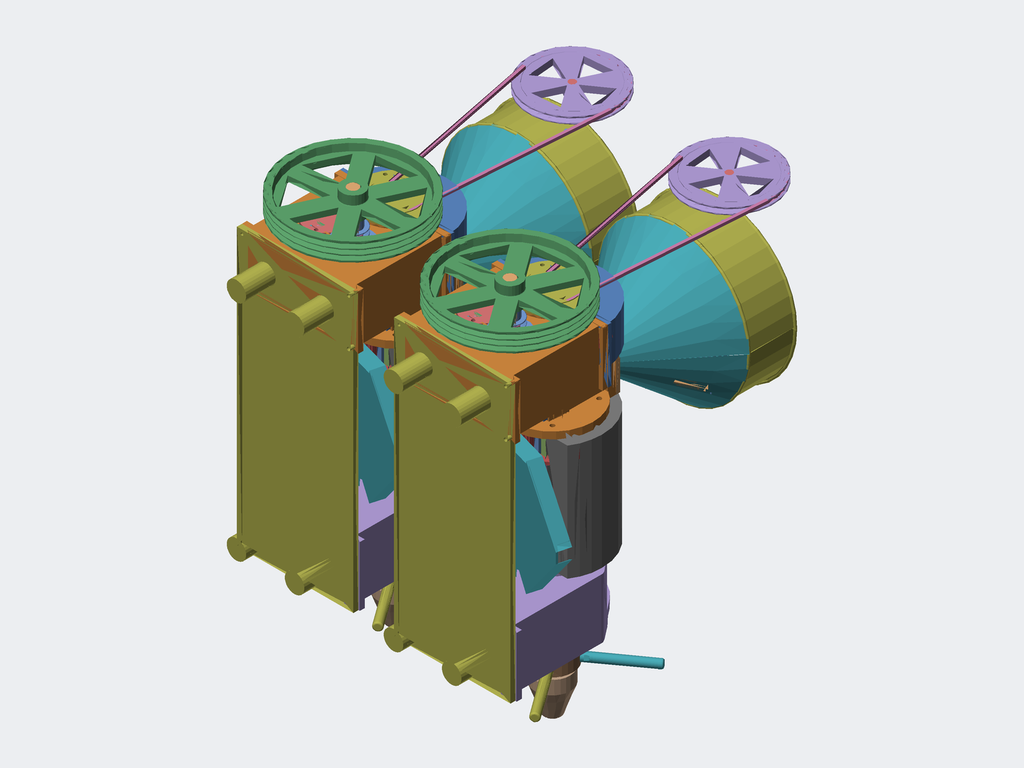Assembly | SolidWorks | 63 different items | 150 placed
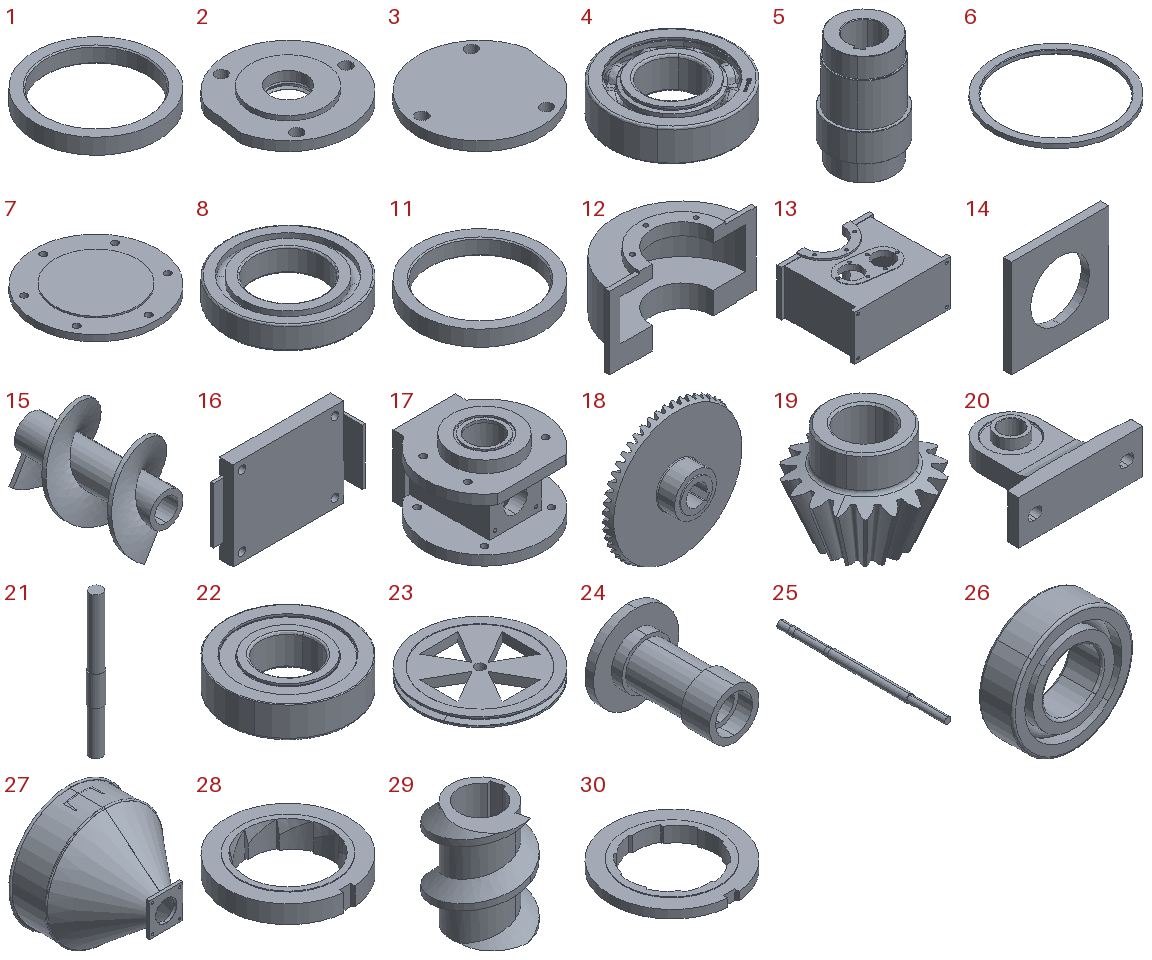Parts list (item | quantity | size | volume | features):
1 | x2 | 55 x 55 x 7 mm | 5462 mm3 | features Revolution 1
2 | x2 | 130.573 x 132 x 19 mm | 150304 mm3 | features HoleWzd 2, Revolution 2, BaseBody 1, Extrusion 1
3 | x6 | 130.573 x 132 x 14 mm | 142005 mm3 | features HoleWzd 2, Extrusion 1, Revolution 1
4 | x4 | 90 x 90 x 23 mm | 82930 mm3 | features BaseBody 14
5 | x2 | 110 x 110 x 178 mm | 973022 mm3 | features BaseBody 1
6 | x1 | 114 x 114 x 4 mm | 9333 mm3 | features Revolution 1
7 | x2 | 240 x 240 x 17.5 mm | 563209 mm3 | features ICE 3, HoleWzd 2, Revolution 1
8 | x4 | 170 x 170 x 32 mm | 443055 mm3 | features BaseBody 1
9 | x2 | - | - | features BaseBody 1
10 | x2 | - | - | features BaseBody 1
11 | x4 | 55 x 55 x 7 mm | 5462 mm3 | features Revolution 1
12 | x2 | 410 x 187 x 210 mm | 2846531 mm3 | features ICE 6, HoleWzd 2, Extrusion 1, RevCut 1
13 | x2 | 430 x 352 x 210 mm | 7645856 mm3 | features ICE 16, HoleWzd 12, Extrusion 1, Fillet 1
14 | x2 | 120 x 10 x 120 mm | 103285 mm3 | features Extrusion 1
15 | x2 | 82 x 130 x 82 mm | 90947 mm3 | features ICE 3, BaseBody 1, HoleWzd 1
16 | x2 | 144 x 31 x 100 mm | 183212 mm3 | features BaseBody 1, Extrusion 1
17 | x2 | 300 x 305 x 198 mm | 5533662 mm3 | features HoleWzd 8, ICE 6, Revolution 2, Extrusion 1
18 | x2 | 160.088 x 42.208 x 160.125 mm | 285045 mm3 | features BaseBody 1
19 | x2 | 61.792 x 61.935 x 51.071 mm | 51754 mm3 | features BaseBody 1
20 | x4 | 142 x 118.08 x 50 mm | 239637 mm3 | features ICE 3, Revolution 3, Fillet 2, BaseBody 1, Chamfer 1, HoleWzd 1
21 | x2 | 28 x 28 x 290 mm | 149846 mm3 | features Revolution 1
22 | x4 | 90 x 90 x 23 mm | 84067 mm3 | features BaseBody 14
23 | x2 | 320 x 320 x 39 mm | 1356183 mm3 | features Fillet 3, ICE 2, Revolution 2, BaseBody 1, HoleWzd 1, RevCut 1
24 | x2 | 120 x 165 x 120 mm | 395872 mm3 | features Revolution 1
25 | x2 | - | - | features ICE 3, RefSurface 1, Revolution 1
26 | x2 | 52 x 15 x 52 mm | 20902 mm3 | features BaseBody 1
27 | x2 | 572 x 466.152 x 572 mm | 1942635 mm3 | features BaseBody 4
28 | x4 | 150 x 149.673 x 31.5 mm | 269452 mm3 | features BaseBody 1, ICE 1
29 | x6 | 95 x 95 x 120 mm | 282927 mm3 | features BaseBody 1, ICE 1, RevCut 1
30 | x6 | 150 x 149.673 x 18.5 mm | 146475 mm3 | features BaseBody 1, ICE 1
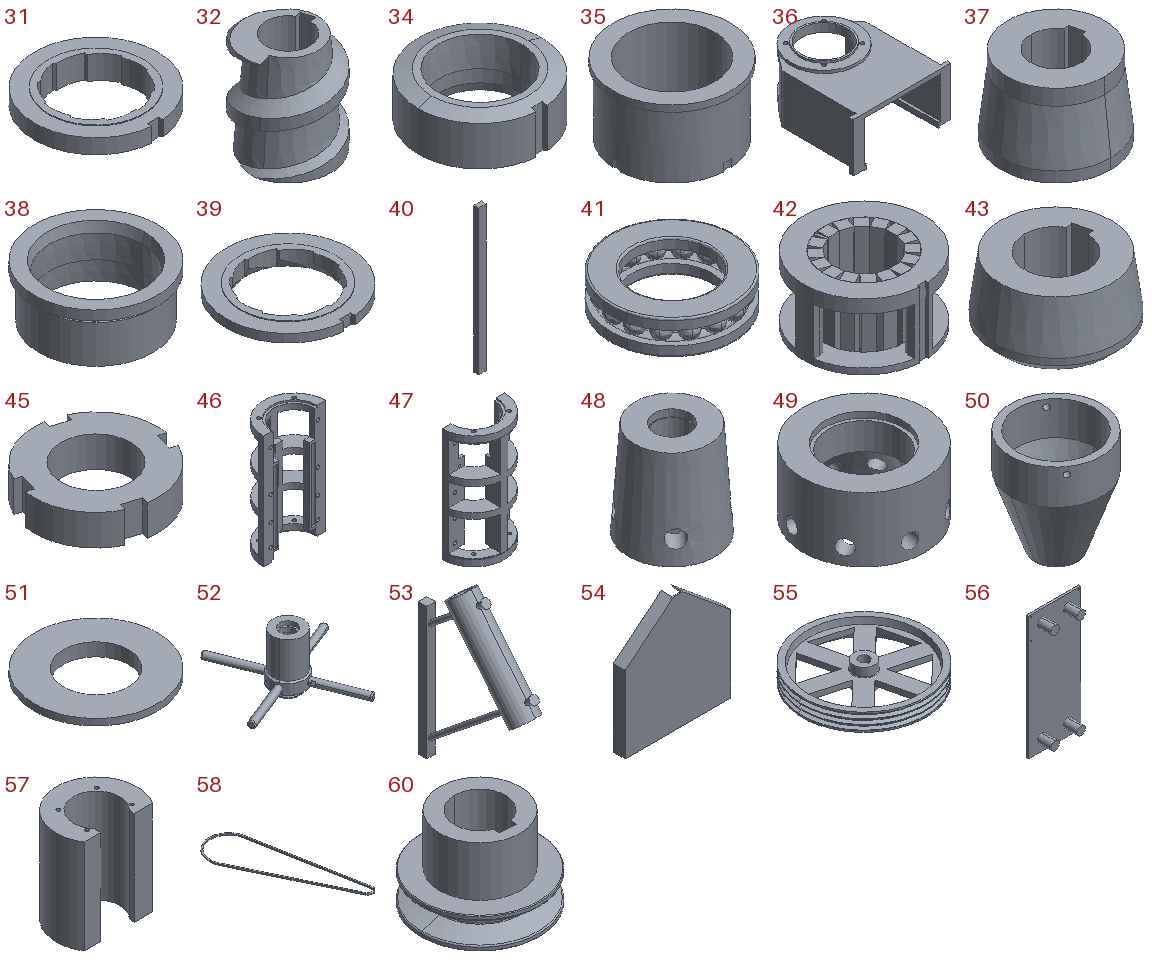31 | x4 | 150 x 149.673 x 28.6 mm | 237488 mm3 | features BaseBody 1, ICE 1
32 | x2 | 95.001 x 95.001 x 109 mm | 363521 mm3 | features BaseBody 1, ICE 1, RevCut 1
33 | x2 | - | - | features BaseBody 1
34 | x2 | 150 x 149.673 x 58.5 mm | 537765 mm3 | features BaseBody 1, ICE 1
35 | x2 | 185 x 185 x 110 mm | 1098272 mm3 | features ICE 5, HoleWzd 1, Revolution 1
36 | x2 | 440 x 502 x 295 mm | 8777626 mm3 | features ICE 17, Fillet 4, HoleWzd 3, Cut 1, Extrusion 1, Revolution 1
37 | x2 | 106 x 106 x 75 mm | 445446 mm3 | features ICE 1, RevCut 1, Revolution 1
38 | x2 | 130 x 130 x 55 mm | 211427 mm3 | features Revolution 1
39 | x4 | 150 x 149.673 x 18.5 mm | 145659 mm3 | features BaseBody 1, ICE 1
40 | x2 | 14 x 9 x 265 mm | 33390 mm3 | features Extrusion 1
41 | x2 | 73 x 73 x 20 mm | 37195 mm3 | features BaseBody 1
42 | x2 | 200 x 199.755 x 123 mm | 1515679 mm3 | features BaseBody 18
43 | x2 | 95 x 95 x 50 mm | 226212 mm3 | features ICE 1, RevCut 1, Revolution 1
44 | x2 | - | - | features BaseBody 1
45 | x2 | 80 x 80 x 20 mm | 64249 mm3 | features Extrusion 1
46 | x1 | 300 x 150 x 550 mm | 5053436 mm3 | features ICE 6, HoleWzd 3, RevCut 3, Revolution 1
47 | x1 | 300 x 150 x 550 mm | 5063192 mm3 | features ICE 19, HoleWzd 4, RevCut 4, BaseBody 1
48 | x2 | 125 x 125 x 135 mm | 1121518 mm3 | features HoleWzd 7, Revolution 1
49 | x2 | 205 x 205 x 108 mm | 1920095 mm3 | features 3DProfileFeature 8, HoleWzd 8, RevCut 1, Revolution 1
50 | x2 | 130 x 130 x 150 mm | 468175 mm3 | features HoleWzd 2, 3DProfileFeature 1, Fillet 1, Revolution 1
51 | x2 | 95 x 95 x 10 mm | 41529 mm3 | features Revolution 1
52 | x2 | 555.753 x 555.753 x 240 mm | 3106019 mm3 | features BaseBody 5
53 | x2 | 45 x 200.096 x 286.61 mm | 222734 mm3 | features ICE 7, Cut 1, Extrusion 1
54 | x2 | 425.348 x 48 x 468.238 mm | 1599795 mm3 | features Cut 1, Extrusion 1, Shell 1
55 | x2 | 470 x 470 x 87 mm | 3518075 mm3 | features ICE 5, Fillet 4, BaseBody 1, RevCut 1
56 | x2 | 430 x 128 x 1020 mm | 9620878 mm3 | features Extrusion 1, ICE 1
57 | x2 | 364.306 x 280.408 x 426 mm | 21434816 mm3 | features Extrusion 1
58 | x2 | 465.093 x 1023 x 10 mm | 233862 mm3 | features ExtruThin 1
59 | x2 | - | - | features ICE 5, BaseBody 1, RefSurface 1, Revolution 1
60 | x2 | 88 x 88 x 60 mm | 133834 mm3 | features Fillet 2, ICE 2, Chamfer 1, RevCut 1, Revolution 1
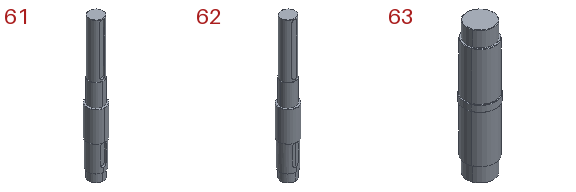61 | x2 | 50 x 50 x 384 mm | 534684 mm3 | features BaseBody 1
62 | x1 | - | - | features ICE 6, RefSurface 2, Chamfer 1, Revolution 1
63 | x2 | 48 x 48 x 200 mm | 297463 mm3 | features BaseBody 1
Mates (type | each side: item.copy, entity, surface, feature):
Coincident | 55.1 face plane Boss-Extrude1 | 61.1 edge
Concentric | 55.1 face cylinder Cut-Revolve1 | 61.1 face cylinder Gearbox assembly-1/1-shaft-1/1-shaft-1-solid1
Parallel | 55.1 face plane Cut-Extrude1 | 61.1 face plane Gearbox assembly-1/1-shaft-1/1-shaft-1-solid1
Concentric | 61.1 face cylinder Gearbox assembly-1/1-shaft-1/1-shaft-1-solid1 | 60.1 face cylinder Cut-Revolve1
Parallel | 61.1 face plane Gearbox assembly-1/1-shaft-1/1-shaft-1-solid1 | 60.1 face plane Cut-Extrude1
Coincident | 55.1 face plane Boss-Extrude2 | 60.1 face plane Boss-Extrude1
Concentric | 13.1 face cylinder M80 clearance hole1 | 61.1 face cylinder Gearbox assembly-1/1-shaft-1/1-shaft-1-solid1
Coincident | 13.1 face plane Boss-Extrude12 | 2.1 face plane Boss-Extrude1
Concentric | 13.1 face cylinder Ø12.0 (12) diameter hole5 | 2.1 face cylinder Ø12.5 (12.5) Diameter Hole1 | 2 times
Concentric | 13.1 face cylinder M80 clearance hole2 | 4.1 face cylinder Gearbox assembly-1/1-shaft-1/1-bearing-gearbox 6308-1-solid11
Coincident | 13.1 face plane Boss-Extrude14 | 4.1 face plane Gearbox assembly-1/1-shaft-1/1-bearing-gearbox 6308-1-solid6
Coincident | 61.1 face plane Gearbox assembly-1/1-shaft-1/1-shaft-1-solid1 | 4.1 face plane Gearbox assembly-1/1-shaft-1/1-bearing-gearbox 6308-1-solid11
Concentric | 13.1 face cylinder M80 clearance hole2 | 4.2 face cylinder Gearbox assembly-1/1-shaft-1/1-bearing-gearbox 6308-1-solid11
Coincident | 13.1 face plane Boss-Extrude13 | 4.2 face plane Gearbox assembly-1/1-shaft-1/1-bearing-gearbox 6308-1-solid6
Coincident | 10.1 face plane Gearbox assembly-1/1-shaft-1/1-small spur gear-1-solid1 | 61.1 face plane Gearbox assembly-1/1-shaft-1/1-shaft-1-solid1
Parallel | 10.1 face plane Gearbox assembly-1/1-shaft-1/1-small spur gear-1-solid1 | 61.1 face plane Gearbox assembly-1/1-shaft-1/1-shaft-1-solid1
Concentric | 10.1 face cylinder Gearbox assembly-1/1-shaft-1/1-small spur gear-1-solid1 | 61.1 face cylinder Gearbox assembly-1/1-shaft-1/1-shaft-1-solid1
Coincident | 1.1 face plane Revolve1 | 4.2 face plane Gearbox assembly-1/1-shaft-1/1-bearing-gearbox 6308-1-solid6
Concentric | 61.1 face cylinder Gearbox assembly-1/1-shaft-1/1-shaft-1-solid1 | 1.1 face cylinder Revolve1
Coincident | 13.1 face plane Boss-Extrude9 | 3.1 face plane Boss-Extrude1
Concentric | 13.1 face cylinder Ø12.0 (12) diameter hole4 | 3.1 face cylinder Ø12.5 (12.5) Diameter Hole1 | 2 times
Concentric | 13.1 face cylinder M80 clearance hole1 | 63.1 face cylinder Gearbox assembly-1/2-shaft-1/2-shaft-1-solid1
Coincident | 13.1 face plane Boss-Extrude12 | 63.1 face plane Gearbox assembly-1/2-shaft-1/2-shaft-1-solid1
Concentric | 13.1 face cylinder M80 clearance hole1 | 22.1 face cylinder Gearbox assembly-1/2-shaft-1/2-bearing-gearbox 6308-1-solid11
Coincident | 13.1 face plane Boss-Extrude14 | 22.1 face plane Gearbox assembly-1/2-shaft-1/2-bearing-gearbox 6308-1-solid6
Concentric | 13.1 face cylinder M80 clearance hole2 | 22.2 face cylinder Gearbox assembly-1/2-shaft-1/2-bearing-gearbox 6308-1-solid11
Coincident | 13.1 face plane Boss-Extrude13 | 22.2 face plane Gearbox assembly-1/2-shaft-1/2-bearing-gearbox 6308-1-solid6
Coincident | 13.1 face plane Boss-Extrude12 | 3.2 face plane Boss-Extrude1
Concentric | 13.1 face cylinder Ø12.0 (12) diameter hole5 | 3.2 face cylinder Ø12.5 (12.5) Diameter Hole1 | 2 times
Coincident | 13.1 face plane Boss-Extrude9 | 3.3 face plane Boss-Extrude1
Concentric | 13.1 face cylinder Ø12.0 (12) diameter hole4 | 3.3 face cylinder Ø12.5 (12.5) Diameter Hole1 | 2 times
Concentric | 63.1 face cylinder Gearbox assembly-1/2-shaft-1/2-shaft-1-solid1 | 11.1 face cylinder Revolve1
Coincident | 11.1 face plane Revolve1 | 22.2 face plane Gearbox assembly-1/2-shaft-1/2-bearing-gearbox 6308-1-solid11
Concentric | 63.1 face cylinder Gearbox assembly-1/2-shaft-1/2-shaft-1-solid1 | 9.1 face cylinder Gearbox assembly-1/2-shaft-1/2-large spur gear-1-solid1
Parallel | 63.1 face plane Gearbox assembly-1/2-shaft-1/2-shaft-1-solid1 | 9.1 face plane Gearbox assembly-1/2-shaft-1/2-large spur gear-1-solid1
Coincident | 11.1 face plane Revolve1 | 9.1 face plane Gearbox assembly-1/2-shaft-1/2-large spur gear-1-solid1
Coincident | 22.1 face plane Gearbox assembly-1/2-shaft-1/2-bearing-gearbox 6308-1-solid11 | 11.2 face plane Revolve1
Coincident | 44.1 face plane Gearbox assembly-1/2-shaft-1/2-small spur gear-1-solid1 | 11.2 face plane Revolve1
Concentric | 63.1 face cylinder Gearbox assembly-1/2-shaft-1/2-shaft-1-solid1 | 44.1 face cylinder Gearbox assembly-1/2-shaft-1/2-small spur gear-1-solid1
Parallel | 63.1 face plane Gearbox assembly-1/2-shaft-1/2-shaft-1-solid1 | 44.1 face plane Gearbox assembly-1/2-shaft-1/2-small spur gear-1-solid1
Coincident | 13.1 face plane Boss-Extrude6 | 7.1 face plane Revolve1
Concentric | 13.1 face cylinder Hole1 | 7.1 face cylinder M90 counterbore hole1
Concentric | 13.1 face cylinder Ø12.0 (12) diameter hole1 | 7.1 face cylinder Ø12.5 (12.5) Diameter Hole1
Coincident | 13.1 face plane Cut-Extrude1 | 8.1 face plane Gearbox assembly-1/3-shaft-2/3-bearing 6219-1-solid1
Concentric | 13.1 face cylinder Hole1 | 8.1 face cylinder Gearbox assembly-1/3-shaft-2/3-bearing 6219-1-solid1
Concentric | 13.1 face cylinder Hole2 | 8.2 face cylinder Gearbox assembly-1/3-shaft-2/3-bearing 6219-1-solid1
Coincident | 13.1 face plane Cut-Extrude1 | 8.2 face plane Gearbox assembly-1/3-shaft-2/3-bearing 6219-1-solid1
Concentric | 5.1 face cylinder Gearbox assembly-1/3-shaft-2/3-shaft-1-solid1 | 8.1 face cylinder Gearbox assembly-1/3-shaft-2/3-bearing 6219-1-solid1
Coincident | 5.1 face plane Gearbox assembly-1/3-shaft-2/3-shaft-1-solid1 | 8.2 face plane Gearbox assembly-1/3-shaft-2/3-bearing 6219-1-solid1
Concentric | 33.1 face cylinder Gearbox assembly-1/3-shaft-2/3-large spur gear-1-solid1 | 5.1 face cylinder Gearbox assembly-1/3-shaft-2/3-shaft-1-solid1
Parallel | 33.1 face plane Gearbox assembly-1/3-shaft-2/3-large spur gear-1-solid1 | 5.1 face plane Gearbox assembly-1/3-shaft-2/3-shaft-1-solid1
Coincident | 33.1 face plane Gearbox assembly-1/3-shaft-2/3-large spur gear-1-solid1 | 5.1 face plane Gearbox assembly-1/3-shaft-2/3-shaft-1-solid1
GearDim | 33.1 select_type:24 | 44.1 select_type:24
Coincident | 12.1 face plane Boss-Extrude1 | 13.1 face plane Boss-Extrude4
Coincident | 12.1 face plane Boss-Extrude1 | 13.1 face plane Boss-Extrude2
Coincident | 12.1 face plane Boss-Extrude1 | 13.1 face plane Boss-Extrude5
Coincident | 20.1 face plane Input3 | 27.1 face plane Hopper-1/Hopper-channel steel 14a-1-solid1
Concentric | 20.1 face cylinder Input3 | 27.1 face cylinder Hopper-1/Hopper-channel steel 14a-1-solid1 | 2 times
Parallel | 20.1 face cylinder Input3 | 27.1 face cylinder Hopper-1/Hopper-channel steel 14a-1-solid1
Coincident | 27.1 face plane Hopper-1/Hopper-channel steel 14a-1-solid1 | 20.2 face plane Input3
Concentric | 27.1 face cylinder Hopper-1/Hopper-channel steel 14a-1-solid1 | 20.2 face cylinder Input3 | 2 times
Concentric | 21.1 face cylinder Revolve1 | 20.2 face cylinder Ø25.0 (25) diameter hole1
Coincident | 21.1 face plane Revolve1 | 20.2 face plane Revolve3
Concentric | 21.1 face cylinder Revolve1 | 23.1 face cylinder Ø25.0 (25) diameter hole1
Coincident | 21.1 face plane Revolve1 | 23.1 face plane Cut-Revolve1
Coincident | 21.1 select_type:24 | 23.1 select_type:24
Coincident | 17.1 face plane Boss-Extrude4 | 27.1 face plane Hopper-1/Hopper-base-1-solid1
Concentric | 17.1 face cylinder Ø10.0 (10) diameter hole1 | 27.1 face cylinder Hopper-1/Hopper-base-1-solid1 | 2 times
Coincident | 16.1 face plane Input3 | 17.1 face plane Boss-Extrude2
Concentric | 16.1 face cylinder Input3 | 17.1 face cylinder Ø8.0 (8) diameter hole1 | 2 times
Concentric | 25.1 face cylinder Revolve1 | 27.1 face cylinder Hopper-1/Hopper-channel steel 14a-1-solid1
Coincident | 18.1 face plane Hopper-1/Hopper-bevel gear assembly-1/Hopper-bevel gear-large gear-1-solid1 | 25.1 face plane Boss-Extrude1
Concentric | 18.1 face cylinder Hopper-1/Hopper-bevel gear assembly-1/Hopper-bevel gear-large gear-1-solid1 | 25.1 face cylinder Boss-Extrude1
Parallel | 18.1 face plane Hopper-1/Hopper-bevel gear assembly-1/Hopper-bevel gear-large gear-1-solid1 | 25.1 face plane Cut-Extrude1
Coincident | 14.1 face plane Boss-Extrude1 | 27.1 face plane Hopper-1/Hopper-channel steel 14a-1-solid1
Parallel | 14.1 edge | 27.1 edge
Concentric | 14.1 face cylinder Boss-Extrude1 | 27.1 face cylinder Hopper-1/Hopper-channel steel 14a-1-solid1
Coincident | 24.1 face plane Revolve1 | 14.1 face plane Boss-Extrude1
Concentric | 24.1 face cylinder Revolve1 | 14.1 face cylinder Boss-Extrude1
Concentric | 21.1 face cylinder Revolve1 | 19.1 face cylinder Hopper-1/Hopper-bevel gear assembly-1/Hopper-bevel gear-small gear-1-solid1
Coincident | 21.1 face plane Revolve1 | 19.1 face plane Hopper-1/Hopper-bevel gear assembly-1/Hopper-bevel gear-small gear-1-solid1
Coincident | 18.1 face plane Hopper-1/Hopper-bevel gear assembly-1/Hopper-bevel gear-large gear-1-solid1 | 24.1 face plane Revolve1
Concentric | 25.1 face cylinder Revolve1 | 26.1 face cylinder Hopper-1/Hopper-auger-1/Hopper-bearing 6205-RS-1-solid1
Coincident | 24.1 face plane Revolve1 | 26.1 face plane Hopper-1/Hopper-auger-1/Hopper-bearing 6205-RS-1-solid1
Concentric | 25.1 face cylinder Boss-Extrude2 | 15.1 face cylinder Ø22.0 (22) diameter hole1
Coincident | 25.1 face plane Revolve1 | 15.1 face plane Boss-Extrude2
Concentric | 8.2 face cylinder Gearbox assembly-1/3-shaft-2/3-bearing 6219-1-solid1 | 17.1 face cylinder M80 counterbore hole1
Coincident | 12.1 face plane Boss-Extrude2 | 17.1 face plane Boss-Extrude3
Concentric | 13.1 face cylinder Ø16.0 (16) diameter hole1 | 17.1 face cylinder Ø16.5 (16.5) diameter hole1
GearDim | 19.1 select_type:24 | 18.1 select_type:24
Coincident | 21.1 select_type:24 | 19.1 select_type:24
Concentric | 5.1 face cylinder Gearbox assembly-1/3-shaft-2/3-shaft-1-solid1 | 59.1 face cylinder Boss-Extrude4 | 2 times
Parallel | 5.1 edge | 59.1 select_type:24
Coincident | 51.1 face plane Revolve1 | 59.1 face plane Boss-Extrude4
Concentric | 51.1 face cylinder Revolve1 | 59.1 face cylinder Boss-Extrude3
Concentric | 32.1 face cylinder Cut-Revolve1 | 59.1 face cylinder Boss-Extrude3
Concentric | 29.1 face cylinder Cut-Revolve1 | 59.1 face cylinder Boss-Extrude3
Coincident | 51.1 face plane Revolve1 | 29.1 face plane Input3
Concentric | 59.1 face cylinder Boss-Extrude3 | 29.2 face cylinder Cut-Revolve1
Parallel | 29.1 edge | 59.1 select_type:24
Coincident | 29.1 face plane Input3 | 29.2 face plane Input3
Lock | 29.1 select_type:0 | 29.2 select_type:0
Concentric | 59.1 face cylinder Boss-Extrude3 | 29.3 face cylinder Cut-Revolve1
Coincident | 29.2 face plane Input3 | 29.3 face plane Input3
Lock | 29.2 select_type:0 | 29.3 select_type:0
Coincident | 32.1 face plane Input3 | 29.3 face plane Input3
Lock | 32.1 select_type:0 | 29.3 select_type:0
Concentric | 43.1 face cylinder Cut-Revolve1 | 59.1 face cylinder Boss-Extrude3
Coincident | 32.1 face plane Input3 | 43.1 face plane Revolve1
Parallel | 43.1 edge | 59.1 select_type:24
Concentric | 38.1 face cone Revolve1 | 59.1 face cylinder Boss-Extrude3
Coincident | 38.1 face plane Revolve1 | 43.1 face plane Revolve1
Concentric | 37.1 face cylinder Cut-Revolve1 | 59.1 face cylinder Boss-Extrude1
Coincident | 37.1 face plane Revolve1 | 43.1 face plane Revolve1
Concentric | 48.1 face cylinder M42 counterbore hole1 | 59.1 face cylinder Boss-Extrude1
Coincident | 37.1 face plane Revolve1 | 48.1 face plane Revolve1
Coincident | 38.1 face plane Revolve1 | 49.1 face plane Revolve1
Concentric | 38.1 face cylinder Revolve1 | 49.1 face cylinder Cut-Revolve1
Concentric | 41.1 face cylinder Press screw-1/Press screw-GB/T 301-1995[thrust ball bearing[51000]51209]-1-solid1 | 59.1 face cylinder Revolve1
Concentric | 52.1 face cylinder Press screw-1/Press screw-adjusting screw-1-solid1 | 59.1 face cylinder Input3
Coincident | 48.1 face plane Revolve1 | 52.1 face plane Press screw-1/Press screw-adjusting screw-1-solid1
Coincident | 52.1 face plane Press screw-1/Press screw-adjusting screw-1-solid1 | 41.1 face plane Press screw-1/Press screw-GB/T 301-1995[thrust ball bearing[51000]51209]-1-solid1
Concentric | 45.1 face cylinder Boss-Extrude1 | 59.1 face cylinder Revolve1
Coincident | 41.1 face plane Press screw-1/Press screw-GB/T 301-1995[thrust ball bearing[51000]51209]-1-solid1 | 45.1 face plane Boss-Extrude1
Concentric | 50.1 face cylinder M100 clearance hole1 | 59.1 face cylinder Revolve1
Coincident | 52.1 edge | 50.1 face plane Revolve1
Concentric | 35.1 face cylinder Hole1 | 52.1 face cylinder Press screw-1/Press screw-adjusting screw-1-solid1
Concentric | 35.1 face cylinder Boss-Extrude1 | 36.1 face cylinder Hole2
Lock | 35.1 select_type:0 | 52.1 select_type:0
Coincident | 35.1 face plane Cut-Extrude3 | 36.1 face plane M10 counterbore hole1
Coincident | 17.1 face plane Boss-Extrude3 | 51.1 face plane Revolve1
Coincident | 17.1 face plane Revolve1 | 42.1 face plane Oil discharge bar-1/Oil discharge bar-strip bar support-1-solid1
Concentric | 17.1 face cylinder M80 counterbore hole1 | 42.1 face cone Oil discharge bar-1/Oil discharge bar-strip bar support-1-solid1
Coincident | 25.1 select_type:24 | 15.1 select_type:24
Coincident | 42.1 face plane Oil discharge bar-1/Oil discharge bar-strip bar support-1-solid1 | 28.1 face plane Three-stage round bar-1/Round bar set-No.4 round bar-1-solid1
Concentric | 59.1 face cylinder Boss-Extrude4 | 28.1 edge
Concentric | 59.1 face cylinder Boss-Extrude4 | 31.1 edge
Concentric | 8.2 edge | 30.1 edge
Concentric | 59.1 face cylinder Boss-Extrude4 | 39.1 edge
Concentric | 59.1 face cylinder Boss-Extrude4 | 34.1 edge
Coincident | 31.1 face plane Three-stage round bar-1/Round bar set-No.3 round bar-2-solid1 | 28.1 face plane Three-stage round bar-1/Round bar set-No.4 round bar-1-solid1 | 2 times
Coincident | 31.1 face plane Cut-Extrude1 | 30.1 face plane Three-stage round bar-1/Round bar set-No.2 round bar-1-solid1
Coincident | 30.1 face plane Cut-Extrude1 | 39.1 face plane Three-stage round bar-1/Round bar set-No.2 round bar outer-1-solid1
Concentric | 59.1 face cylinder Boss-Extrude4 | 30.2 edge
Concentric | 59.1 face cylinder Boss-Extrude4 | 31.2 edge
Concentric | 59.1 face cylinder Boss-Extrude4 | 39.2 edge
Concentric | 59.1 face cylinder Boss-Extrude4 | 28.2 edge
Coincident | 39.1 face plane Cut-Extrude1 | 28.2 face plane Three-stage round bar-1/Round bar set-No.4 round bar-1-solid1
Coincident | 31.2 face plane Three-stage round bar-1/Round bar set-No.3 round bar-2-solid1 | 28.2 face plane Three-stage round bar-1/Round bar set-No.4 round bar-1-solid1 | 2 times
Coincident | 31.2 face plane Cut-Extrude1 | 30.2 face plane Three-stage round bar-1/Round bar set-No.2 round bar-1-solid1
Coincident | 30.2 face plane Cut-Extrude1 | 39.2 face plane Three-stage round bar-1/Round bar set-No.2 round bar outer-1-solid1
Concentric | 59.1 face cylinder Boss-Extrude4 | 30.3 edge
Coincident | 39.2 face plane Cut-Extrude1 | 30.3 face plane Three-stage round bar-1/Round bar set-No.2 round bar-1-solid1
Coincident | 34.1 face plane Three-stage round bar-1/Round bar set-No.5 round bar-1-solid1 | 30.3 face plane Cut-Extrude1
Parallel | 42.1 face plane Oil discharge bar-1/Oil discharge bar-strip bar support-1-solid1 | 28.1 face plane Three-stage round bar-1/Round bar set-No.4 round bar-1-solid1
Coincident | 31.1 face plane Three-stage round bar-1/Round bar set-No.3 round bar-2-solid1 | 30.1 face plane Three-stage round bar-1/Round bar set-No.2 round bar-1-solid1
Coincident | 30.1 face plane Three-stage round bar-1/Round bar set-No.2 round bar-1-solid1 | 39.1 face plane Three-stage round bar-1/Round bar set-No.2 round bar outer-1-solid1
Coincident | 39.1 face plane Three-stage round bar-1/Round bar set-No.2 round bar outer-1-solid1 | 28.2 face plane Three-stage round bar-1/Round bar set-No.4 round bar-1-solid1
Coincident | 31.2 face plane Three-stage round bar-1/Round bar set-No.3 round bar-2-solid1 | 30.2 face plane Three-stage round bar-1/Round bar set-No.2 round bar-1-solid1
Coincident | 30.2 face plane Three-stage round bar-1/Round bar set-No.2 round bar-1-solid1 | 39.2 face plane Three-stage round bar-1/Round bar set-No.2 round bar outer-1-solid1
Coincident | 34.1 face plane Three-stage round bar-1/Round bar set-No.5 round bar-1-solid1 | 39.2 face plane Three-stage round bar-1/Round bar set-No.2 round bar outer-1-solid1
Coincident | 39.2 face plane Three-stage round bar-1/Round bar set-No.2 round bar outer-1-solid1 | 30.3 face plane Three-stage round bar-1/Round bar set-No.2 round bar-1-solid1
Coincident | 28.1 face plane Three-stage round bar-1/Round bar set-No.4 round bar-1-solid1 | 40.1 face plane Boss-Extrude1
Coincident | 28.1 edge | 40.1 edge
Coincident | 49.1 face plane Revolve1 | 40.1 face plane Boss-Extrude1
Parallel | 13.1 edge | 36.1 edge
Parallel | 13.1 edge | 40.1 edge
Concentric | 60.1 face cylinder Revolve1 | 58.1 face cylinder Thin-wall extrude1
Concentric | 23.1 face cylinder Fixed part | 58.1 face cylinder Thin-wall extrude1
GearDim | 23.1 select_type:24 | 60.1 select_type:24
Coincident | 17.1 face plane Boss-Extrude1 | 57.1 face plane Boss-Extrude1
Concentric | 17.1 face cylinder Ø16.0 (16) diameter hole1 | 57.1 face cylinder Boss-Extrude1 | 2 times
Concentric | 13.1 face cylinder Ø11.0 (11) diameter hole1 | 56.1 face cylinder Boss-Extrude1 | 2 times
Coincident | 13.1 face plane Boss-Extrude3 | 56.1 face plane Boss-Extrude1
Coincident | 57.1 edge | 54.1 edge
Concentric | 25.1 face cylinder Revolve1 | 53.1 face cylinder Boss-Extrude4
Parallel | 18.1 select_type:24 | 53.1 select_type:24
GearDim | 9.1 select_type:24 | 10.1 select_type:24